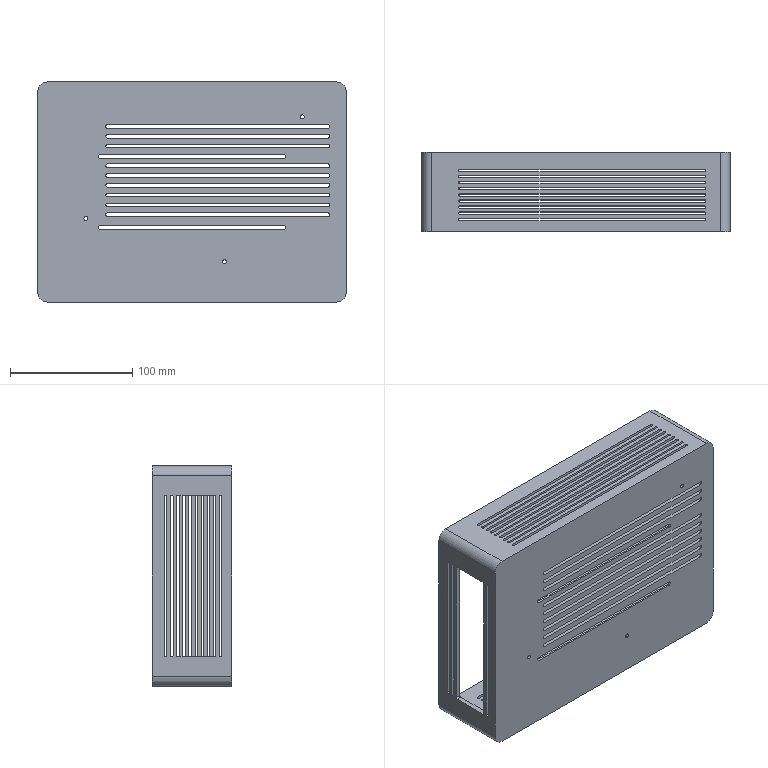Part | SolidWorks | features ICE 11, Fillet 5, MoveFace 5, HoleWzd 2, Cut 1, Extrusion 1 | 1 solid | 300 faces | box 252 x 65 x 180 mm | volume 401045 mm3 | cylinder 173 | plane 105 | cone 18 | sphere 4 | commonest cylinder face diameters 2 x97 2.5 x32 3 x18 6 x8 3.3 x6 3.2 x4